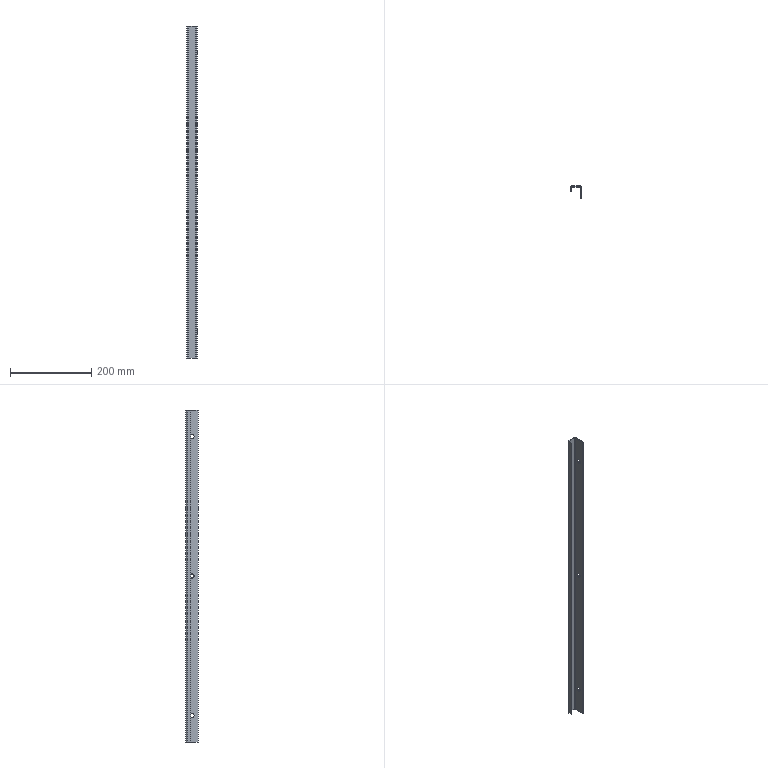Part | STEP file | 750078281 | 1 solid | 20 faces | box 25 x 30 x 817 mm | volume 98215 mm3 | cylinder 10 | plane 10 | commonest cylinder face diameters 10.5 x6 4 x2 8 x2
STEP:
#1=CARTESIAN_POINT('',(-2.,15.,348.75));
#2=VERTEX_POINT('',#1);
#3=CARTESIAN_POINT('',(-2.,15.,338.25));
#4=VERTEX_POINT('',#3);
#5=CARTESIAN_POINT('',(-2.,15.,343.5));
#6=DIRECTION('',(1.,0.,0.));
#7=DIRECTION('',(0.,0.,-1.));
#8=AXIS2_PLACEMENT_3D('',#5,#6,#7);
#9=CIRCLE('',#8,5.25);
#10=EDGE_CURVE('',#2,#4,#9,.T.);
#11=ORIENTED_EDGE('',*,*,#10,.F.);
#12=CARTESIAN_POINT('',(0.,15.,348.75));
#13=VERTEX_POINT('',#12);
#14=CARTESIAN_POINT('',(-2.,15.,348.75));
#15=DIRECTION('',(1.,0.,0.));
#16=VECTOR('',#15,1000.);
#17=LINE('',#14,#16);
#18=EDGE_CURVE('',#2,#13,#17,.T.);
#19=ORIENTED_EDGE('',*,*,#18,.T.);
#20=CARTESIAN_POINT('',(0.,15.,338.25));
#21=VERTEX_POINT('',#20);
#22=CARTESIAN_POINT('',(0.,15.,343.5));
#23=DIRECTION('',(-1.,0.,0.));
#24=DIRECTION('',(0.,0.,-1.));
#25=AXIS2_PLACEMENT_3D('',#22,#23,#24);
#26=CIRCLE('',#25,5.25);
#27=EDGE_CURVE('',#21,#13,#26,.T.);
#28=ORIENTED_EDGE('',*,*,#27,.F.);
#29=CARTESIAN_POINT('',(-2.,15.,338.25));
#30=DIRECTION('',(1.,0.,0.));
#31=VECTOR('',#30,1000.);
#32=LINE('',#29,#31);
#33=EDGE_CURVE('',#4,#21,#32,.T.);
#34=ORIENTED_EDGE('',*,*,#33,.F.);
#35=EDGE_LOOP('',(#11,#19,#28,#34));
#36=FACE_OUTER_BOUND('',#35,.T.);
#37=CARTESIAN_POINT('',(-2.,15.,343.5));
#38=DIRECTION('',(1.,0.,0.));
#39=DIRECTION('',(0.,0.,-1.));
#40=AXIS2_PLACEMENT_3D('',#37,#38,#39);
#41=CYLINDRICAL_SURFACE('',#40,5.25);
#42=ADVANCED_FACE('',(#36),#41,.F.);
#43=CARTESIAN_POINT('',(-2.,15.,5.25));
#44=VERTEX_POINT('',#43);
#45=CARTESIAN_POINT('',(-2.,15.,-5.25));
#46=VERTEX_POINT('',#45);
#47=CARTESIAN_POINT('',(-2.,15.,0.));
#48=DIRECTION('',(1.,0.,0.));
#49=DIRECTION('',(0.,0.,-1.));
#50=AXIS2_PLACEMENT_3D('',#47,#48,#49);
#51=CIRCLE('',#50,5.25);
#52=EDGE_CURVE('',#44,#46,#51,.T.);
#53=ORIENTED_EDGE('',*,*,#52,.F.);
#54=CARTESIAN_POINT('',(0.,15.,5.25));
#55=VERTEX_POINT('',#54);
#56=CARTESIAN_POINT('',(-2.,15.,5.25));
#57=DIRECTION('',(1.,0.,0.));
#58=VECTOR('',#57,1000.);
#59=LINE('',#56,#58);
#60=EDGE_CURVE('',#44,#55,#59,.T.);
#61=ORIENTED_EDGE('',*,*,#60,.T.);
#62=CARTESIAN_POINT('',(0.,15.,-5.25));
#63=VERTEX_POINT('',#62);
#64=CARTESIAN_POINT('',(0.,15.,0.));
#65=DIRECTION('',(-1.,0.,0.));
#66=DIRECTION('',(0.,0.,-1.));
#67=AXIS2_PLACEMENT_3D('',#64,#65,#66);
#68=CIRCLE('',#67,5.25);
#69=EDGE_CURVE('',#63,#55,#68,.T.);
#70=ORIENTED_EDGE('',*,*,#69,.F.);
#71=CARTESIAN_POINT('',(-2.,15.,-5.25));
#72=DIRECTION('',(1.,0.,0.));
#73=VECTOR('',#72,1000.);
#74=LINE('',#71,#73);
#75=EDGE_CURVE('',#46,#63,#74,.T.);
#76=ORIENTED_EDGE('',*,*,#75,.F.);
#77=EDGE_LOOP('',(#53,#61,#70,#76));
#78=FACE_OUTER_BOUND('',#77,.T.);
#79=CARTESIAN_POINT('',(-2.,15.,0.));
#80=DIRECTION('',(1.,0.,0.));
#81=DIRECTION('',(0.,0.,-1.));
#82=AXIS2_PLACEMENT_3D('',#79,#80,#81);
#83=CYLINDRICAL_SURFACE('',#82,5.25);
#84=ADVANCED_FACE('',(#78),#83,.F.);
#85=CARTESIAN_POINT('',(-2.,15.,-338.25));
#86=VERTEX_POINT('',#85);
#87=CARTESIAN_POINT('',(-2.,15.,-348.75));
#88=VERTEX_POINT('',#87);
#89=CARTESIAN_POINT('',(-2.,15.,-343.5));
#90=DIRECTION('',(1.,0.,0.));
#91=DIRECTION('',(0.,0.,-1.));
#92=AXIS2_PLACEMENT_3D('',#89,#90,#91);
#93=CIRCLE('',#92,5.25);
#94=EDGE_CURVE('',#86,#88,#93,.T.);
#95=ORIENTED_EDGE('',*,*,#94,.F.);
#96=CARTESIAN_POINT('',(0.,15.,-338.25));
#97=VERTEX_POINT('',#96);
#98=CARTESIAN_POINT('',(-2.,15.,-338.25));
#99=DIRECTION('',(1.,0.,0.));
#100=VECTOR('',#99,1000.);
#101=LINE('',#98,#100);
#102=EDGE_CURVE('',#86,#97,#101,.T.);
#103=ORIENTED_EDGE('',*,*,#102,.T.);
#104=CARTESIAN_POINT('',(0.,15.,-348.75));
#105=VERTEX_POINT('',#104);
#106=CARTESIAN_POINT('',(0.,15.,-343.5));
#107=DIRECTION('',(-1.,0.,0.));
#108=DIRECTION('',(0.,0.,-1.));
#109=AXIS2_PLACEMENT_3D('',#106,#107,#108);
#110=CIRCLE('',#109,5.25);
#111=EDGE_CURVE('',#105,#97,#110,.T.);
#112=ORIENTED_EDGE('',*,*,#111,.F.);
#113=CARTESIAN_POINT('',(-2.,15.,-348.75));
#114=DIRECTION('',(1.,0.,0.));
#115=VECTOR('',#114,1000.);
#116=LINE('',#113,#115);
#117=EDGE_CURVE('',#88,#105,#116,.T.);
#118=ORIENTED_EDGE('',*,*,#117,.F.);
#119=EDGE_LOOP('',(#95,#103,#112,#118));
#120=FACE_OUTER_BOUND('',#119,.T.);
#121=CARTESIAN_POINT('',(-2.,15.,-343.5));
#122=DIRECTION('',(1.,0.,0.));
#123=DIRECTION('',(0.,0.,-1.));
#124=AXIS2_PLACEMENT_3D('',#121,#122,#123);
#125=CYLINDRICAL_SURFACE('',#124,5.25);
#126=ADVANCED_FACE('',(#120),#125,.F.);
#127=CARTESIAN_POINT('',(0.,26.,408.5));
#128=VERTEX_POINT('',#127);
#129=CARTESIAN_POINT('',(0.,0.,408.5));
#130=VERTEX_POINT('',#129);
#131=CARTESIAN_POINT('',(0.,30.,408.5));
#132=DIRECTION('',(0.,-1.,0.));
#133=VECTOR('',#132,1000.);
#134=LINE('',#131,#133);
#135=EDGE_CURVE('',#128,#130,#134,.T.);
#136=ORIENTED_EDGE('',*,*,#135,.T.);
#137=CARTESIAN_POINT('',(0.,0.,-408.5));
#138=VERTEX_POINT('',#137);
#139=CARTESIAN_POINT('',(0.,0.,408.5));
#140=DIRECTION('',(0.,0.,-1.));
#141=VECTOR('',#140,1000.);
#142=LINE('',#139,#141);
#143=EDGE_CURVE('',#130,#138,#142,.T.);
#144=ORIENTED_EDGE('',*,*,#143,.T.);
#145=CARTESIAN_POINT('',(0.,26.,-408.5));
#146=VERTEX_POINT('',#145);
#147=CARTESIAN_POINT('',(0.,30.,-408.5));
#148=DIRECTION('',(0.,1.,0.));
#149=VECTOR('',#148,1000.);
#150=LINE('',#147,#149);
#151=EDGE_CURVE('',#138,#146,#150,.T.);
#152=ORIENTED_EDGE('',*,*,#151,.T.);
#153=CARTESIAN_POINT('',(0.,26.,408.5));
#154=DIRECTION('',(0.,0.,1.));
#155=VECTOR('',#154,1000.);
#156=LINE('',#153,#155);
#157=EDGE_CURVE('',#146,#128,#156,.T.);
#158=ORIENTED_EDGE('',*,*,#157,.T.);
#159=EDGE_LOOP('',(#136,#144,#152,#158));
#160=FACE_OUTER_BOUND('',#159,.T.);
#161=ORIENTED_EDGE('',*,*,#27,.T.);
#162=CARTESIAN_POINT('',(0.,15.,343.5));
#163=DIRECTION('',(-1.,0.,0.));
#164=DIRECTION('',(0.,0.,-1.));
#165=AXIS2_PLACEMENT_3D('',#162,#163,#164);
#166=CIRCLE('',#165,5.25);
#167=EDGE_CURVE('',#13,#21,#166,.T.);
#168=ORIENTED_EDGE('',*,*,#167,.T.);
#169=EDGE_LOOP('',(#161,#168));
#170=FACE_BOUND('',#169,.T.);
#171=ORIENTED_EDGE('',*,*,#69,.T.);
#172=CARTESIAN_POINT('',(0.,15.,0.));
#173=DIRECTION('',(-1.,0.,0.));
#174=DIRECTION('',(0.,0.,-1.));
#175=AXIS2_PLACEMENT_3D('',#172,#173,#174);
#176=CIRCLE('',#175,5.25);
#177=EDGE_CURVE('',#55,#63,#176,.T.);
#178=ORIENTED_EDGE('',*,*,#177,.T.);
#179=EDGE_LOOP('',(#171,#178));
#180=FACE_BOUND('',#179,.T.);
#181=ORIENTED_EDGE('',*,*,#111,.T.);
#182=CARTESIAN_POINT('',(0.,15.,-343.5));
#183=DIRECTION('',(-1.,0.,0.));
#184=DIRECTION('',(0.,0.,-1.));
#185=AXIS2_PLACEMENT_3D('',#182,#183,#184);
#186=CIRCLE('',#185,5.25);
#187=EDGE_CURVE('',#97,#105,#186,.T.);
#188=ORIENTED_EDGE('',*,*,#187,.T.);
#189=EDGE_LOOP('',(#181,#188));
#190=FACE_BOUND('',#189,.T.);
#191=CARTESIAN_POINT('',(0.,30.,408.5));
#192=DIRECTION('',(1.,0.,0.));
#193=DIRECTION('',(0.,0.,-1.));
#194=AXIS2_PLACEMENT_3D('',#191,#192,#193);
#195=PLANE('',#194);
#196=ADVANCED_FACE('',(#160,#170,#180,#190),#195,.T.);
#197=CARTESIAN_POINT('',(-2.,0.,-408.5));
#198=VERTEX_POINT('',#197);
#199=CARTESIAN_POINT('',(0.,0.,-408.5));
#200=DIRECTION('',(1.,0.,0.));
#201=VECTOR('',#200,1000.);
#202=LINE('',#199,#201);
#203=EDGE_CURVE('',#198,#138,#202,.T.);
#204=ORIENTED_EDGE('',*,*,#203,.T.);
#205=ORIENTED_EDGE('',*,*,#143,.F.);
#206=CARTESIAN_POINT('',(-2.,0.,408.5));
#207=VERTEX_POINT('',#206);
#208=CARTESIAN_POINT('',(0.,0.,408.5));
#209=DIRECTION('',(-1.,0.,0.));
#210=VECTOR('',#209,1000.);
#211=LINE('',#208,#210);
#212=EDGE_CURVE('',#130,#207,#211,.T.);
#213=ORIENTED_EDGE('',*,*,#212,.T.);
#214=CARTESIAN_POINT('',(-2.,0.,408.5));
#215=DIRECTION('',(0.,0.,-1.));
#216=VECTOR('',#215,1000.);
#217=LINE('',#214,#216);
#218=EDGE_CURVE('',#207,#198,#217,.T.);
#219=ORIENTED_EDGE('',*,*,#218,.T.);
#220=EDGE_LOOP('',(#204,#205,#213,#219));
#221=FACE_OUTER_BOUND('',#220,.T.);
#222=CARTESIAN_POINT('',(0.,0.,408.5));
#223=DIRECTION('',(0.,-1.,0.));
#224=DIRECTION('',(0.,0.,-1.));
#225=AXIS2_PLACEMENT_3D('',#222,#223,#224);
#226=PLANE('',#225);
#227=ADVANCED_FACE('',(#221),#226,.T.);
#228=CARTESIAN_POINT('',(-2.,26.,408.5));
#229=VERTEX_POINT('',#228);
#230=CARTESIAN_POINT('',(-2.,30.,408.5));
#231=DIRECTION('',(0.,-1.,0.));
#232=VECTOR('',#231,1000.);
#233=LINE('',#230,#232);
#234=EDGE_CURVE('',#229,#207,#233,.T.);
#235=ORIENTED_EDGE('',*,*,#234,.T.);
#236=ORIENTED_EDGE('',*,*,#212,.F.);
#237=ORIENTED_EDGE('',*,*,#135,.F.);
#238=CARTESIAN_POINT('',(-4.,30.,408.5));
#239=VERTEX_POINT('',#238);
#240=CARTESIAN_POINT('',(-4.,26.,408.5));
#241=DIRECTION('',(0.,0.,1.));
#242=DIRECTION('',(-1.,0.,0.));
#243=AXIS2_PLACEMENT_3D('',#240,#241,#242);
#244=CIRCLE('',#243,4.);
#245=EDGE_CURVE('',#128,#239,#244,.T.);
#246=ORIENTED_EDGE('',*,*,#245,.T.);
#247=CARTESIAN_POINT('',(-21.,30.,408.5));
#248=VERTEX_POINT('',#247);
#249=CARTESIAN_POINT('',(0.,30.,408.5));
#250=DIRECTION('',(-1.,0.,0.));
#251=VECTOR('',#250,1000.);
#252=LINE('',#249,#251);
#253=EDGE_CURVE('',#239,#248,#252,.T.);
#254=ORIENTED_EDGE('',*,*,#253,.T.);
#255=CARTESIAN_POINT('',(-25.,26.,408.5));
#256=VERTEX_POINT('',#255);
#257=CARTESIAN_POINT('',(-21.,26.,408.5));
#258=DIRECTION('',(0.,0.,1.));
#259=DIRECTION('',(-1.,0.,0.));
#260=AXIS2_PLACEMENT_3D('',#257,#258,#259);
#261=CIRCLE('',#260,4.);
#262=EDGE_CURVE('',#248,#256,#261,.T.);
#263=ORIENTED_EDGE('',*,*,#262,.T.);
#264=CARTESIAN_POINT('',(-25.,18.,408.5));
#265=VERTEX_POINT('',#264);
#266=CARTESIAN_POINT('',(-25.,30.,408.5));
#267=DIRECTION('',(0.,-1.,0.));
#268=VECTOR('',#267,1000.);
#269=LINE('',#266,#268);
#270=EDGE_CURVE('',#256,#265,#269,.T.);
#271=ORIENTED_EDGE('',*,*,#270,.T.);
#272=CARTESIAN_POINT('',(-23.,18.,408.5));
#273=VERTEX_POINT('',#272);
#274=CARTESIAN_POINT('',(0.,18.,408.5));
#275=DIRECTION('',(1.,0.,0.));
#276=VECTOR('',#275,1000.);
#277=LINE('',#274,#276);
#278=EDGE_CURVE('',#265,#273,#277,.T.);
#279=ORIENTED_EDGE('',*,*,#278,.T.);
#280=CARTESIAN_POINT('',(-23.,26.,408.5));
#281=VERTEX_POINT('',#280);
#282=CARTESIAN_POINT('',(-23.,30.,408.5));
#283=DIRECTION('',(0.,1.,0.));
#284=VECTOR('',#283,1000.);
#285=LINE('',#282,#284);
#286=EDGE_CURVE('',#273,#281,#285,.T.);
#287=ORIENTED_EDGE('',*,*,#286,.T.);
#288=CARTESIAN_POINT('',(-21.,28.,408.5));
#289=VERTEX_POINT('',#288);
#290=CARTESIAN_POINT('',(-21.,26.,408.5));
#291=DIRECTION('',(0.,0.,-1.));
#292=DIRECTION('',(-1.,0.,0.));
#293=AXIS2_PLACEMENT_3D('',#290,#291,#292);
#294=CIRCLE('',#293,2.);
#295=EDGE_CURVE('',#281,#289,#294,.T.);
#296=ORIENTED_EDGE('',*,*,#295,.T.);
#297=CARTESIAN_POINT('',(-4.,28.,408.5));
#298=VERTEX_POINT('',#297);
#299=CARTESIAN_POINT('',(0.,28.,408.5));
#300=DIRECTION('',(1.,0.,0.));
#301=VECTOR('',#300,1000.);
#302=LINE('',#299,#301);
#303=EDGE_CURVE('',#289,#298,#302,.T.);
#304=ORIENTED_EDGE('',*,*,#303,.T.);
#305=CARTESIAN_POINT('',(-4.,26.,408.5));
#306=DIRECTION('',(0.,0.,-1.));
#307=DIRECTION('',(-1.,0.,0.));
#308=AXIS2_PLACEMENT_3D('',#305,#306,#307);
#309=CIRCLE('',#308,2.);
#310=EDGE_CURVE('',#298,#229,#309,.T.);
#311=ORIENTED_EDGE('',*,*,#310,.T.);
#312=EDGE_LOOP('',(#235,#236,#237,#246,#254,#263,#271,#279,#287,#296,#304,#311));
#313=FACE_OUTER_BOUND('',#312,.T.);
#314=CARTESIAN_POINT('',(0.,30.,408.5));
#315=DIRECTION('',(0.,0.,1.));
#316=DIRECTION('',(1.,0.,0.));
#317=AXIS2_PLACEMENT_3D('',#314,#315,#316);
#318=PLANE('',#317);
#319=ADVANCED_FACE('',(#313),#318,.T.);
#320=ORIENTED_EDGE('',*,*,#245,.F.);
#321=ORIENTED_EDGE('',*,*,#157,.F.);
#322=CARTESIAN_POINT('',(-4.,30.,-408.5));
#323=VERTEX_POINT('',#322);
#324=CARTESIAN_POINT('',(-4.,26.,-408.5));
#325=DIRECTION('',(0.,0.,1.));
#326=DIRECTION('',(-1.,0.,0.));
#327=AXIS2_PLACEMENT_3D('',#324,#325,#326);
#328=CIRCLE('',#327,4.);
#329=EDGE_CURVE('',#146,#323,#328,.T.);
#330=ORIENTED_EDGE('',*,*,#329,.T.);
#331=CARTESIAN_POINT('',(-4.,30.,408.5));
#332=DIRECTION('',(0.,0.,1.));
#333=VECTOR('',#332,1000.);
#334=LINE('',#331,#333);
#335=EDGE_CURVE('',#323,#239,#334,.T.);
#336=ORIENTED_EDGE('',*,*,#335,.T.);
#337=EDGE_LOOP('',(#320,#321,#330,#336));
#338=FACE_OUTER_BOUND('',#337,.T.);
#339=CARTESIAN_POINT('',(-4.,26.,408.5));
#340=DIRECTION('',(0.,0.,-1.));
#341=DIRECTION('',(-1.,0.,0.));
#342=AXIS2_PLACEMENT_3D('',#339,#340,#341);
#343=CYLINDRICAL_SURFACE('',#342,4.);
#344=ADVANCED_FACE('',(#338),#343,.T.);
#345=CARTESIAN_POINT('',(-21.,30.,-408.5));
#346=VERTEX_POINT('',#345);
#347=CARTESIAN_POINT('',(-25.,26.,-408.5));
#348=VERTEX_POINT('',#347);
#349=CARTESIAN_POINT('',(-21.,26.,-408.5));
#350=DIRECTION('',(0.,0.,1.));
#351=DIRECTION('',(-1.,0.,0.));
#352=AXIS2_PLACEMENT_3D('',#349,#350,#351);
#353=CIRCLE('',#352,4.);
#354=EDGE_CURVE('',#346,#348,#353,.T.);
#355=ORIENTED_EDGE('',*,*,#354,.F.);
#356=CARTESIAN_POINT('',(-25.,30.,-408.5));
#357=DIRECTION('',(-1.,0.,0.));
#358=VECTOR('',#357,1000.);
#359=LINE('',#356,#358);
#360=EDGE_CURVE('',#323,#346,#359,.T.);
#361=ORIENTED_EDGE('',*,*,#360,.F.);
#362=ORIENTED_EDGE('',*,*,#329,.F.);
#363=ORIENTED_EDGE('',*,*,#151,.F.);
#364=ORIENTED_EDGE('',*,*,#203,.F.);
#365=CARTESIAN_POINT('',(-2.,26.,-408.5));
#366=VERTEX_POINT('',#365);
#367=CARTESIAN_POINT('',(-2.,18.,-408.5));
#368=DIRECTION('',(0.,-1.,0.));
#369=VECTOR('',#368,1000.);
#370=LINE('',#367,#369);
#371=EDGE_CURVE('',#366,#198,#370,.T.);
#372=ORIENTED_EDGE('',*,*,#371,.F.);
#373=CARTESIAN_POINT('',(-4.,28.,-408.5));
#374=VERTEX_POINT('',#373);
#375=CARTESIAN_POINT('',(-4.,26.,-408.5));
#376=DIRECTION('',(0.,0.,-1.));
#377=DIRECTION('',(-1.,0.,0.));
#378=AXIS2_PLACEMENT_3D('',#375,#376,#377);
#379=CIRCLE('',#378,2.);
#380=EDGE_CURVE('',#374,#366,#379,.T.);
#381=ORIENTED_EDGE('',*,*,#380,.F.);
#382=CARTESIAN_POINT('',(-21.,28.,-408.5));
#383=VERTEX_POINT('',#382);
#384=CARTESIAN_POINT('',(-25.,28.,-408.5));
#385=DIRECTION('',(1.,0.,0.));
#386=VECTOR('',#385,1000.);
#387=LINE('',#384,#386);
#388=EDGE_CURVE('',#383,#374,#387,.T.);
#389=ORIENTED_EDGE('',*,*,#388,.F.);
#390=CARTESIAN_POINT('',(-23.,26.,-408.5));
#391=VERTEX_POINT('',#390);
#392=CARTESIAN_POINT('',(-21.,26.,-408.5));
#393=DIRECTION('',(0.,0.,-1.));
#394=DIRECTION('',(-1.,0.,0.));
#395=AXIS2_PLACEMENT_3D('',#392,#393,#394);
#396=CIRCLE('',#395,2.);
#397=EDGE_CURVE('',#391,#383,#396,.T.);
#398=ORIENTED_EDGE('',*,*,#397,.F.);
#399=CARTESIAN_POINT('',(-23.,18.,-408.5));
#400=VERTEX_POINT('',#399);
#401=CARTESIAN_POINT('',(-23.,18.,-408.5));
#402=DIRECTION('',(0.,1.,0.));
#403=VECTOR('',#402,1000.);
#404=LINE('',#401,#403);
#405=EDGE_CURVE('',#400,#391,#404,.T.);
#406=ORIENTED_EDGE('',*,*,#405,.F.);
#407=CARTESIAN_POINT('',(-25.,18.,-408.5));
#408=VERTEX_POINT('',#407);
#409=CARTESIAN_POINT('',(-25.,18.,-408.5));
#410=DIRECTION('',(1.,0.,0.));
#411=VECTOR('',#410,1000.);
#412=LINE('',#409,#411);
#413=EDGE_CURVE('',#408,#400,#412,.T.);
#414=ORIENTED_EDGE('',*,*,#413,.F.);
#415=CARTESIAN_POINT('',(-25.,18.,-408.5));
#416=DIRECTION('',(0.,-1.,0.));
#417=VECTOR('',#416,1000.);
#418=LINE('',#415,#417);
#419=EDGE_CURVE('',#348,#408,#418,.T.);
#420=ORIENTED_EDGE('',*,*,#419,.F.);
#421=EDGE_LOOP('',(#355,#361,#362,#363,#364,#372,#381,#389,#398,#406,#414,#420));
#422=FACE_OUTER_BOUND('',#421,.T.);
#423=CARTESIAN_POINT('',(-25.,18.,-408.5));
#424=DIRECTION('',(0.,0.,1.));
#425=DIRECTION('',(1.,0.,0.));
#426=AXIS2_PLACEMENT_3D('',#423,#424,#425);
#427=PLANE('',#426);
#428=ADVANCED_FACE('',(#422),#427,.F.);
#429=ORIENTED_EDGE('',*,*,#18,.F.);
#430=CARTESIAN_POINT('',(-2.,15.,343.5));
#431=DIRECTION('',(1.,0.,0.));
#432=DIRECTION('',(0.,0.,-1.));
#433=AXIS2_PLACEMENT_3D('',#430,#431,#432);
#434=CIRCLE('',#433,5.25);
#435=EDGE_CURVE('',#4,#2,#434,.T.);
#436=ORIENTED_EDGE('',*,*,#435,.F.);
#437=ORIENTED_EDGE('',*,*,#33,.T.);
#438=ORIENTED_EDGE('',*,*,#167,.F.);
#439=EDGE_LOOP('',(#429,#436,#437,#438));
#440=FACE_OUTER_BOUND('',#439,.T.);
#441=CARTESIAN_POINT('',(-2.,15.,343.5));
#442=DIRECTION('',(1.,0.,0.));
#443=DIRECTION('',(0.,0.,-1.));
#444=AXIS2_PLACEMENT_3D('',#441,#442,#443);
#445=CYLINDRICAL_SURFACE('',#444,5.25);
#446=ADVANCED_FACE('',(#440),#445,.F.);
#447=ORIENTED_EDGE('',*,*,#60,.F.);
#448=CARTESIAN_POINT('',(-2.,15.,0.));
#449=DIRECTION('',(1.,0.,0.));
#450=DIRECTION('',(0.,0.,-1.));
#451=AXIS2_PLACEMENT_3D('',#448,#449,#450);
#452=CIRCLE('',#451,5.25);
#453=EDGE_CURVE('',#46,#44,#452,.T.);
#454=ORIENTED_EDGE('',*,*,#453,.F.);
#455=ORIENTED_EDGE('',*,*,#75,.T.);
#456=ORIENTED_EDGE('',*,*,#177,.F.);
#457=EDGE_LOOP('',(#447,#454,#455,#456));
#458=FACE_OUTER_BOUND('',#457,.T.);
#459=CARTESIAN_POINT('',(-2.,15.,0.));
#460=DIRECTION('',(1.,0.,0.));
#461=DIRECTION('',(0.,0.,-1.));
#462=AXIS2_PLACEMENT_3D('',#459,#460,#461);
#463=CYLINDRICAL_SURFACE('',#462,5.25);
#464=ADVANCED_FACE('',(#458),#463,.F.);
#465=ORIENTED_EDGE('',*,*,#102,.F.);
#466=CARTESIAN_POINT('',(-2.,15.,-343.5));
#467=DIRECTION('',(1.,0.,0.));
#468=DIRECTION('',(0.,0.,-1.));
#469=AXIS2_PLACEMENT_3D('',#466,#467,#468);
#470=CIRCLE('',#469,5.25);
#471=EDGE_CURVE('',#88,#86,#470,.T.);
#472=ORIENTED_EDGE('',*,*,#471,.F.);
#473=ORIENTED_EDGE('',*,*,#117,.T.);
#474=ORIENTED_EDGE('',*,*,#187,.F.);
#475=EDGE_LOOP('',(#465,#472,#473,#474));
#476=FACE_OUTER_BOUND('',#475,.T.);
#477=CARTESIAN_POINT('',(-2.,15.,-343.5));
#478=DIRECTION('',(1.,0.,0.));
#479=DIRECTION('',(0.,0.,-1.));
#480=AXIS2_PLACEMENT_3D('',#477,#478,#479);
#481=CYLINDRICAL_SURFACE('',#480,5.25);
#482=ADVANCED_FACE('',(#476),#481,.F.);
#483=ORIENTED_EDGE('',*,*,#218,.F.);
#484=ORIENTED_EDGE('',*,*,#234,.F.);
#485=CARTESIAN_POINT('',(-2.,26.,408.5));
#486=DIRECTION('',(0.,0.,1.));
#487=VECTOR('',#486,1000.);
#488=LINE('',#485,#487);
#489=EDGE_CURVE('',#366,#229,#488,.T.);
#490=ORIENTED_EDGE('',*,*,#489,.F.);
#491=ORIENTED_EDGE('',*,*,#371,.T.);
#492=EDGE_LOOP('',(#483,#484,#490,#491));
#493=FACE_OUTER_BOUND('',#492,.T.);
#494=ORIENTED_EDGE('',*,*,#435,.T.);
#495=ORIENTED_EDGE('',*,*,#10,.T.);
#496=EDGE_LOOP('',(#494,#495));
#497=FACE_BOUND('',#496,.T.);
#498=ORIENTED_EDGE('',*,*,#453,.T.);
#499=ORIENTED_EDGE('',*,*,#52,.T.);
#500=EDGE_LOOP('',(#498,#499));
#501=FACE_BOUND('',#500,.T.);
#502=ORIENTED_EDGE('',*,*,#471,.T.);
#503=ORIENTED_EDGE('',*,*,#94,.T.);
#504=EDGE_LOOP('',(#502,#503));
#505=FACE_BOUND('',#504,.T.);
#506=CARTESIAN_POINT('',(-2.,30.,408.5));
#507=DIRECTION('',(1.,0.,0.));
#508=DIRECTION('',(0.,0.,-1.));
#509=AXIS2_PLACEMENT_3D('',#506,#507,#508);
#510=PLANE('',#509);
#511=ADVANCED_FACE('',(#493,#497,#501,#505),#510,.F.);
#512=ORIENTED_EDGE('',*,*,#489,.T.);
#513=ORIENTED_EDGE('',*,*,#310,.F.);
#514=CARTESIAN_POINT('',(-4.,28.,408.5));
#515=DIRECTION('',(0.,0.,1.));
#516=VECTOR('',#515,1000.);
#517=LINE('',#514,#516);
#518=EDGE_CURVE('',#374,#298,#517,.T.);
#519=ORIENTED_EDGE('',*,*,#518,.F.);
#520=ORIENTED_EDGE('',*,*,#380,.T.);
#521=EDGE_LOOP('',(#512,#513,#519,#520));
#522=FACE_OUTER_BOUND('',#521,.T.);
#523=CARTESIAN_POINT('',(-4.,26.,408.5));
#524=DIRECTION('',(0.,0.,-1.));
#525=DIRECTION('',(-1.,0.,0.));
#526=AXIS2_PLACEMENT_3D('',#523,#524,#525);
#527=CYLINDRICAL_SURFACE('',#526,2.);
#528=ADVANCED_FACE('',(#522),#527,.F.);
#529=ORIENTED_EDGE('',*,*,#518,.T.);
#530=ORIENTED_EDGE('',*,*,#303,.F.);
#531=CARTESIAN_POINT('',(-21.,28.,408.5));
#532=DIRECTION('',(0.,0.,1.));
#533=VECTOR('',#532,1000.);
#534=LINE('',#531,#533);
#535=EDGE_CURVE('',#383,#289,#534,.T.);
#536=ORIENTED_EDGE('',*,*,#535,.F.);
#537=ORIENTED_EDGE('',*,*,#388,.T.);
#538=EDGE_LOOP('',(#529,#530,#536,#537));
#539=FACE_OUTER_BOUND('',#538,.T.);
#540=CARTESIAN_POINT('',(-25.,28.,408.5));
#541=DIRECTION('',(0.,1.,0.));
#542=DIRECTION('',(0.,0.,1.));
#543=AXIS2_PLACEMENT_3D('',#540,#541,#542);
#544=PLANE('',#543);
#545=ADVANCED_FACE('',(#539),#544,.F.);
#546=ORIENTED_EDGE('',*,*,#535,.T.);
#547=ORIENTED_EDGE('',*,*,#295,.F.);
#548=CARTESIAN_POINT('',(-23.,26.,408.5));
#549=DIRECTION('',(0.,0.,1.));
#550=VECTOR('',#549,1000.);
#551=LINE('',#548,#550);
#552=EDGE_CURVE('',#391,#281,#551,.T.);
#553=ORIENTED_EDGE('',*,*,#552,.F.);
#554=ORIENTED_EDGE('',*,*,#397,.T.);
#555=EDGE_LOOP('',(#546,#547,#553,#554));
#556=FACE_OUTER_BOUND('',#555,.T.);
#557=CARTESIAN_POINT('',(-21.,26.,408.5));
#558=DIRECTION('',(0.,0.,-1.));
#559=DIRECTION('',(-1.,0.,0.));
#560=AXIS2_PLACEMENT_3D('',#557,#558,#559);
#561=CYLINDRICAL_SURFACE('',#560,2.);
#562=ADVANCED_FACE('',(#556),#561,.F.);
#563=ORIENTED_EDGE('',*,*,#552,.T.);
#564=ORIENTED_EDGE('',*,*,#286,.F.);
#565=CARTESIAN_POINT('',(-23.,18.,408.5));
#566=DIRECTION('',(0.,0.,1.));
#567=VECTOR('',#566,1000.);
#568=LINE('',#565,#567);
#569=EDGE_CURVE('',#400,#273,#568,.T.);
#570=ORIENTED_EDGE('',*,*,#569,.F.);
#571=ORIENTED_EDGE('',*,*,#405,.T.);
#572=EDGE_LOOP('',(#563,#564,#570,#571));
#573=FACE_OUTER_BOUND('',#572,.T.);
#574=CARTESIAN_POINT('',(-23.,18.,408.5));
#575=DIRECTION('',(-1.,0.,0.));
#576=DIRECTION('',(0.,0.,1.));
#577=AXIS2_PLACEMENT_3D('',#574,#575,#576);
#578=PLANE('',#577);
#579=ADVANCED_FACE('',(#573),#578,.F.);
#580=ORIENTED_EDGE('',*,*,#278,.F.);
#581=CARTESIAN_POINT('',(-25.,18.,408.5));
#582=DIRECTION('',(0.,0.,1.));
#583=VECTOR('',#582,1000.);
#584=LINE('',#581,#583);
#585=EDGE_CURVE('',#408,#265,#584,.T.);
#586=ORIENTED_EDGE('',*,*,#585,.F.);
#587=ORIENTED_EDGE('',*,*,#413,.T.);
#588=ORIENTED_EDGE('',*,*,#569,.T.);
#589=EDGE_LOOP('',(#580,#586,#587,#588));
#590=FACE_OUTER_BOUND('',#589,.T.);
#591=CARTESIAN_POINT('',(-25.,18.,408.5));
#592=DIRECTION('',(0.,1.,0.));
#593=DIRECTION('',(0.,0.,1.));
#594=AXIS2_PLACEMENT_3D('',#591,#592,#593);
#595=PLANE('',#594);
#596=ADVANCED_FACE('',(#590),#595,.F.);
#597=ORIENTED_EDGE('',*,*,#270,.F.);
#598=CARTESIAN_POINT('',(-25.,26.,408.5));
#599=DIRECTION('',(0.,0.,-1.));
#600=VECTOR('',#599,1000.);
#601=LINE('',#598,#600);
#602=EDGE_CURVE('',#256,#348,#601,.T.);
#603=ORIENTED_EDGE('',*,*,#602,.T.);
#604=ORIENTED_EDGE('',*,*,#419,.T.);
#605=ORIENTED_EDGE('',*,*,#585,.T.);
#606=EDGE_LOOP('',(#597,#603,#604,#605));
#607=FACE_OUTER_BOUND('',#606,.T.);
#608=CARTESIAN_POINT('',(-25.,18.,408.5));
#609=DIRECTION('',(-1.,0.,0.));
#610=DIRECTION('',(0.,0.,1.));
#611=AXIS2_PLACEMENT_3D('',#608,#609,#610);
#612=PLANE('',#611);
#613=ADVANCED_FACE('',(#607),#612,.T.);
#614=ORIENTED_EDGE('',*,*,#262,.F.);
#615=CARTESIAN_POINT('',(-21.,30.,408.5));
#616=DIRECTION('',(0.,0.,-1.));
#617=VECTOR('',#616,1000.);
#618=LINE('',#615,#617);
#619=EDGE_CURVE('',#248,#346,#618,.T.);
#620=ORIENTED_EDGE('',*,*,#619,.T.);
#621=ORIENTED_EDGE('',*,*,#354,.T.);
#622=ORIENTED_EDGE('',*,*,#602,.F.);
#623=EDGE_LOOP('',(#614,#620,#621,#622));
#624=FACE_OUTER_BOUND('',#623,.T.);
#625=CARTESIAN_POINT('',(-21.,26.,408.5));
#626=DIRECTION('',(0.,0.,-1.));
#627=DIRECTION('',(-1.,0.,0.));
#628=AXIS2_PLACEMENT_3D('',#625,#626,#627);
#629=CYLINDRICAL_SURFACE('',#628,4.);
#630=ADVANCED_FACE('',(#624),#629,.T.);
#631=ORIENTED_EDGE('',*,*,#253,.F.);
#632=ORIENTED_EDGE('',*,*,#335,.F.);
#633=ORIENTED_EDGE('',*,*,#360,.T.);
#634=ORIENTED_EDGE('',*,*,#619,.F.);
#635=EDGE_LOOP('',(#631,#632,#633,#634));
#636=FACE_OUTER_BOUND('',#635,.T.);
#637=CARTESIAN_POINT('',(-25.,30.,408.5));
#638=DIRECTION('',(0.,1.,0.));
#639=DIRECTION('',(0.,0.,1.));
#640=AXIS2_PLACEMENT_3D('',#637,#638,#639);
#641=PLANE('',#640);
#642=ADVANCED_FACE('',(#636),#641,.T.);
#643=CLOSED_SHELL('',(#42,#84,#126,#196,#227,#319,#344,#428,#446,#464,#482,#511,#528,#545,#562,#579,#596,#613,#630,#642));
#644=MANIFOLD_SOLID_BREP('',#643);
#645=CARTESIAN_POINT('',(0.,0.,0.));
#646=DIRECTION('',(0.,0.,1.));
#647=DIRECTION('',(1.,0.,0.));
#648=AXIS2_PLACEMENT_3D('',#645,#646,#647);
#649=(LENGTH_UNIT()NAMED_UNIT(*)SI_UNIT(.MILLI.,.METRE.));
#650=UNCERTAINTY_MEASURE_WITH_UNIT(LENGTH_MEASURE(0.00001),#649,'','');
#651=(NAMED_UNIT(*)PLANE_ANGLE_UNIT()SI_UNIT($,.RADIAN.));
#652=(NAMED_UNIT(*)SI_UNIT($,.STERADIAN.)SOLID_ANGLE_UNIT());
#653=(GEOMETRIC_REPRESENTATION_CONTEXT(3)GLOBAL_UNCERTAINTY_ASSIGNED_CONTEXT((#650))GLOBAL_UNIT_ASSIGNED_CONTEXT((#649,#651,#652))REPRESENTATION_CONTEXT('',''));
#654=ADVANCED_BREP_SHAPE_REPRESENTATION('',(#644,#648),#653);